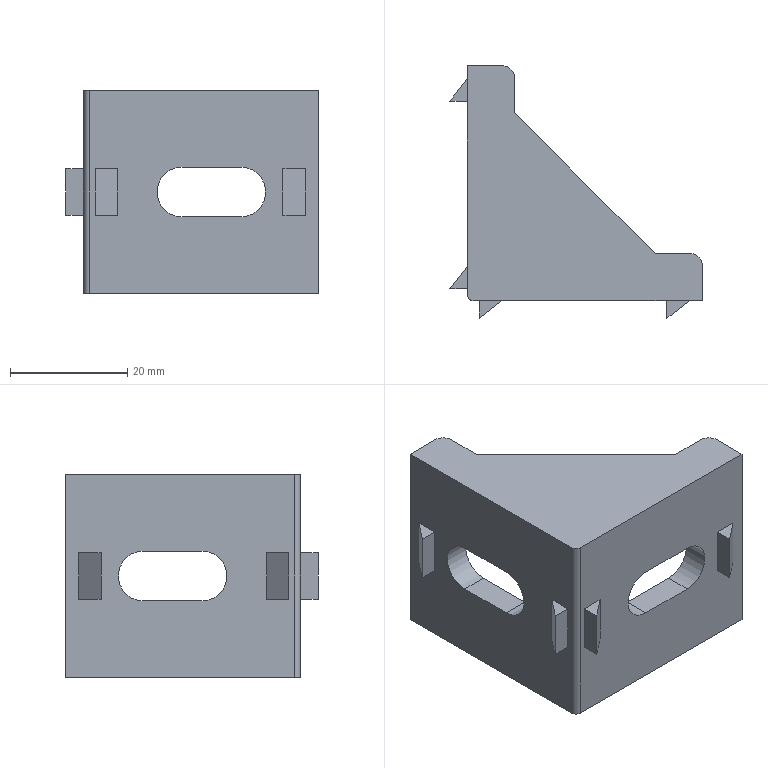Part | SolidWorks | features BaseBody 1 | 1 solid | 45 faces | box 43 x 43 x 34.5 mm | volume 13756 mm3 | plane 36 | cylinder 9 | commonest cylinder face diameters 4 x4 8.5 x4 2 x1
STEP:
#1=CARTESIAN_POINT('',(5.8,0.,-21.25));
#2=VERTEX_POINT('',#1);
#3=CARTESIAN_POINT('',(5.8,0.,-13.25));
#4=VERTEX_POINT('',#3);
#5=CARTESIAN_POINT('',(5.8,0.,-21.25));
#6=DIRECTION('',(0.,0.,1.));
#7=VECTOR('',#6,1000.);
#8=LINE('',#5,#7);
#9=EDGE_CURVE('',#2,#4,#8,.T.);
#10=ORIENTED_EDGE('',*,*,#9,.F.);
#11=CARTESIAN_POINT('',(2.,0.,-21.25));
#12=VERTEX_POINT('',#11);
#13=CARTESIAN_POINT('',(5.8,0.,-21.25));
#14=DIRECTION('',(1.,0.,0.));
#15=VECTOR('',#14,1000.);
#16=LINE('',#13,#15);
#17=EDGE_CURVE('',#12,#2,#16,.T.);
#18=ORIENTED_EDGE('',*,*,#17,.F.);
#19=CARTESIAN_POINT('',(2.,0.,-13.25));
#20=VERTEX_POINT('',#19);
#21=CARTESIAN_POINT('',(2.,0.,-21.25));
#22=DIRECTION('',(0.,0.,1.));
#23=VECTOR('',#22,1000.);
#24=LINE('',#21,#23);
#25=EDGE_CURVE('',#12,#20,#24,.T.);
#26=ORIENTED_EDGE('',*,*,#25,.T.);
#27=CARTESIAN_POINT('',(5.8,0.,-13.25));
#28=DIRECTION('',(1.,0.,0.));
#29=VECTOR('',#28,1000.);
#30=LINE('',#27,#29);
#31=EDGE_CURVE('',#20,#4,#30,.T.);
#32=ORIENTED_EDGE('',*,*,#31,.T.);
#33=EDGE_LOOP('',(#10,#18,#26,#32));
#34=FACE_BOUND('',#33,.T.);
#35=CARTESIAN_POINT('',(16.8,0.,-13.));
#36=VERTEX_POINT('',#35);
#37=CARTESIAN_POINT('',(16.8,0.,-21.5));
#38=VERTEX_POINT('',#37);
#39=CARTESIAN_POINT('',(16.8,0.,-17.25));
#40=DIRECTION('',(0.,-1.,0.));
#41=DIRECTION('',(0.,0.,-1.));
#42=AXIS2_PLACEMENT_3D('',#39,#40,#41);
#43=CIRCLE('',#42,4.25);
#44=EDGE_CURVE('',#36,#38,#43,.T.);
#45=ORIENTED_EDGE('',*,*,#44,.F.);
#46=CARTESIAN_POINT('',(26.8,0.,-13.));
#47=VERTEX_POINT('',#46);
#48=CARTESIAN_POINT('',(0.,0.,-13.));
#49=DIRECTION('',(-1.,0.,0.));
#50=VECTOR('',#49,1000.);
#51=LINE('',#48,#50);
#52=EDGE_CURVE('',#47,#36,#51,.T.);
#53=ORIENTED_EDGE('',*,*,#52,.F.);
#54=CARTESIAN_POINT('',(26.8,0.,-21.5));
#55=VERTEX_POINT('',#54);
#56=CARTESIAN_POINT('',(26.8,0.,-17.25));
#57=DIRECTION('',(0.,-1.,0.));
#58=DIRECTION('',(0.,0.,-1.));
#59=AXIS2_PLACEMENT_3D('',#56,#57,#58);
#60=CIRCLE('',#59,4.25);
#61=EDGE_CURVE('',#55,#47,#60,.T.);
#62=ORIENTED_EDGE('',*,*,#61,.F.);
#63=CARTESIAN_POINT('',(0.,0.,-21.5));
#64=DIRECTION('',(1.,0.,0.));
#65=VECTOR('',#64,1000.);
#66=LINE('',#63,#65);
#67=EDGE_CURVE('',#38,#55,#66,.T.);
#68=ORIENTED_EDGE('',*,*,#67,.F.);
#69=EDGE_LOOP('',(#45,#53,#62,#68));
#70=FACE_BOUND('',#69,.T.);
#71=CARTESIAN_POINT('',(1.,0.,0.));
#72=VERTEX_POINT('',#71);
#73=CARTESIAN_POINT('',(40.,0.,0.));
#74=VERTEX_POINT('',#73);
#75=CARTESIAN_POINT('',(0.,0.,0.));
#76=DIRECTION('',(1.,0.,0.));
#77=VECTOR('',#76,1000.);
#78=LINE('',#75,#77);
#79=EDGE_CURVE('',#72,#74,#78,.T.);
#80=ORIENTED_EDGE('',*,*,#79,.F.);
#81=CARTESIAN_POINT('',(1.,0.,-34.5));
#82=VERTEX_POINT('',#81);
#83=CARTESIAN_POINT('',(1.,0.,-34.5));
#84=DIRECTION('',(0.,0.,-1.));
#85=VECTOR('',#84,1000.);
#86=LINE('',#83,#85);
#87=EDGE_CURVE('',#72,#82,#86,.T.);
#88=ORIENTED_EDGE('',*,*,#87,.T.);
#89=CARTESIAN_POINT('',(40.,0.,-34.5));
#90=VERTEX_POINT('',#89);
#91=CARTESIAN_POINT('',(0.,0.,-34.5));
#92=DIRECTION('',(1.,0.,0.));
#93=VECTOR('',#92,1000.);
#94=LINE('',#91,#93);
#95=EDGE_CURVE('',#82,#90,#94,.T.);
#96=ORIENTED_EDGE('',*,*,#95,.T.);
#97=CARTESIAN_POINT('',(40.,0.,-34.5));
#98=DIRECTION('',(0.,0.,1.));
#99=VECTOR('',#98,1000.);
#100=LINE('',#97,#99);
#101=EDGE_CURVE('',#90,#74,#100,.T.);
#102=ORIENTED_EDGE('',*,*,#101,.T.);
#103=EDGE_LOOP('',(#80,#88,#96,#102));
#104=FACE_OUTER_BOUND('',#103,.T.);
#105=CARTESIAN_POINT('',(37.8,0.,-21.25));
#106=VERTEX_POINT('',#105);
#107=CARTESIAN_POINT('',(37.8,0.,-13.25));
#108=VERTEX_POINT('',#107);
#109=CARTESIAN_POINT('',(37.8,0.,-21.25));
#110=DIRECTION('',(0.,0.,1.));
#111=VECTOR('',#110,1000.);
#112=LINE('',#109,#111);
#113=EDGE_CURVE('',#106,#108,#112,.T.);
#114=ORIENTED_EDGE('',*,*,#113,.F.);
#115=CARTESIAN_POINT('',(34.,0.,-21.25));
#116=VERTEX_POINT('',#115);
#117=CARTESIAN_POINT('',(34.,0.,-21.25));
#118=DIRECTION('',(1.,0.,0.));
#119=VECTOR('',#118,1000.);
#120=LINE('',#117,#119);
#121=EDGE_CURVE('',#116,#106,#120,.T.);
#122=ORIENTED_EDGE('',*,*,#121,.F.);
#123=CARTESIAN_POINT('',(34.,0.,-13.25));
#124=VERTEX_POINT('',#123);
#125=CARTESIAN_POINT('',(34.,0.,-21.25));
#126=DIRECTION('',(0.,0.,1.));
#127=VECTOR('',#126,1000.);
#128=LINE('',#125,#127);
#129=EDGE_CURVE('',#116,#124,#128,.T.);
#130=ORIENTED_EDGE('',*,*,#129,.T.);
#131=CARTESIAN_POINT('',(34.,0.,-13.25));
#132=DIRECTION('',(1.,0.,0.));
#133=VECTOR('',#132,1000.);
#134=LINE('',#131,#133);
#135=EDGE_CURVE('',#124,#108,#134,.T.);
#136=ORIENTED_EDGE('',*,*,#135,.T.);
#137=EDGE_LOOP('',(#114,#122,#130,#136));
#138=FACE_BOUND('',#137,.T.);
#139=CARTESIAN_POINT('',(0.,0.,-34.5));
#140=DIRECTION('',(0.,-1.,0.));
#141=DIRECTION('',(0.,0.,-1.));
#142=AXIS2_PLACEMENT_3D('',#139,#140,#141);
#143=PLANE('',#142);
#144=ADVANCED_FACE('',(#34,#70,#104,#138),#143,.T.);
#145=CARTESIAN_POINT('',(4.5,26.8,-21.5));
#146=VERTEX_POINT('',#145);
#147=CARTESIAN_POINT('',(4.5,26.8,-13.));
#148=VERTEX_POINT('',#147);
#149=CARTESIAN_POINT('',(4.5,26.8,-17.25));
#150=DIRECTION('',(1.,0.,0.));
#151=DIRECTION('',(0.,0.,-1.));
#152=AXIS2_PLACEMENT_3D('',#149,#150,#151);
#153=CIRCLE('',#152,4.25);
#154=EDGE_CURVE('',#146,#148,#153,.T.);
#155=ORIENTED_EDGE('',*,*,#154,.F.);
#156=CARTESIAN_POINT('',(4.5,16.8,-21.5));
#157=VERTEX_POINT('',#156);
#158=CARTESIAN_POINT('',(4.5,26.8,-21.5));
#159=DIRECTION('',(0.,1.,0.));
#160=VECTOR('',#159,1000.);
#161=LINE('',#158,#160);
#162=EDGE_CURVE('',#157,#146,#161,.T.);
#163=ORIENTED_EDGE('',*,*,#162,.F.);
#164=CARTESIAN_POINT('',(4.5,16.8,-13.));
#165=VERTEX_POINT('',#164);
#166=CARTESIAN_POINT('',(4.5,16.8,-17.25));
#167=DIRECTION('',(1.,0.,0.));
#168=DIRECTION('',(0.,0.,-1.));
#169=AXIS2_PLACEMENT_3D('',#166,#167,#168);
#170=CIRCLE('',#169,4.25);
#171=EDGE_CURVE('',#165,#157,#170,.T.);
#172=ORIENTED_EDGE('',*,*,#171,.F.);
#173=CARTESIAN_POINT('',(4.5,26.8,-13.));
#174=DIRECTION('',(0.,-1.,0.));
#175=VECTOR('',#174,1000.);
#176=LINE('',#173,#175);
#177=EDGE_CURVE('',#148,#165,#176,.T.);
#178=ORIENTED_EDGE('',*,*,#177,.F.);
#179=EDGE_LOOP('',(#155,#163,#172,#178));
#180=FACE_BOUND('',#179,.T.);
#181=CARTESIAN_POINT('',(4.5,4.5,-31.5));
#182=VERTEX_POINT('',#181);
#183=CARTESIAN_POINT('',(4.5,4.5,-3.));
#184=VERTEX_POINT('',#183);
#185=CARTESIAN_POINT('',(4.5,4.5,-34.5));
#186=DIRECTION('',(0.,0.,1.));
#187=VECTOR('',#186,1000.);
#188=LINE('',#185,#187);
#189=EDGE_CURVE('',#182,#184,#188,.T.);
#190=ORIENTED_EDGE('',*,*,#189,.F.);
#191=CARTESIAN_POINT('',(4.5,40.,-31.5));
#192=VERTEX_POINT('',#191);
#193=CARTESIAN_POINT('',(4.5,40.,-31.5));
#194=DIRECTION('',(0.,-1.,0.));
#195=VECTOR('',#194,1000.);
#196=LINE('',#193,#195);
#197=EDGE_CURVE('',#192,#182,#196,.T.);
#198=ORIENTED_EDGE('',*,*,#197,.F.);
#199=CARTESIAN_POINT('',(4.5,40.,-3.));
#200=VERTEX_POINT('',#199);
#201=CARTESIAN_POINT('',(4.5,40.,-34.5));
#202=DIRECTION('',(0.,0.,1.));
#203=VECTOR('',#202,1000.);
#204=LINE('',#201,#203);
#205=EDGE_CURVE('',#192,#200,#204,.T.);
#206=ORIENTED_EDGE('',*,*,#205,.T.);
#207=CARTESIAN_POINT('',(4.5,40.,-3.));
#208=DIRECTION('',(0.,-1.,0.));
#209=VECTOR('',#208,1000.);
#210=LINE('',#207,#209);
#211=EDGE_CURVE('',#200,#184,#210,.T.);
#212=ORIENTED_EDGE('',*,*,#211,.T.);
#213=EDGE_LOOP('',(#190,#198,#206,#212));
#214=FACE_OUTER_BOUND('',#213,.T.);
#215=CARTESIAN_POINT('',(4.5,4.5,-34.5));
#216=DIRECTION('',(1.,0.,0.));
#217=DIRECTION('',(0.,0.,-1.));
#218=AXIS2_PLACEMENT_3D('',#215,#216,#217);
#219=PLANE('',#218);
#220=ADVANCED_FACE('',(#180,#214),#219,.T.);
#221=CARTESIAN_POINT('',(16.8,4.5,-21.5));
#222=VERTEX_POINT('',#221);
#223=CARTESIAN_POINT('',(16.8,4.5,-13.));
#224=VERTEX_POINT('',#223);
#225=CARTESIAN_POINT('',(16.8,4.5,-17.25));
#226=DIRECTION('',(0.,1.,0.));
#227=DIRECTION('',(0.,0.,1.));
#228=AXIS2_PLACEMENT_3D('',#225,#226,#227);
#229=CIRCLE('',#228,4.25);
#230=EDGE_CURVE('',#222,#224,#229,.T.);
#231=ORIENTED_EDGE('',*,*,#230,.F.);
#232=CARTESIAN_POINT('',(26.8,4.5,-21.5));
#233=VERTEX_POINT('',#232);
#234=CARTESIAN_POINT('',(16.8,4.5,-21.5));
#235=DIRECTION('',(-1.,0.,0.));
#236=VECTOR('',#235,1000.);
#237=LINE('',#234,#236);
#238=EDGE_CURVE('',#233,#222,#237,.T.);
#239=ORIENTED_EDGE('',*,*,#238,.F.);
#240=CARTESIAN_POINT('',(26.8,4.5,-13.));
#241=VERTEX_POINT('',#240);
#242=CARTESIAN_POINT('',(26.8,4.5,-17.25));
#243=DIRECTION('',(0.,1.,0.));
#244=DIRECTION('',(0.,0.,1.));
#245=AXIS2_PLACEMENT_3D('',#242,#243,#244);
#246=CIRCLE('',#245,4.25);
#247=EDGE_CURVE('',#241,#233,#246,.T.);
#248=ORIENTED_EDGE('',*,*,#247,.F.);
#249=CARTESIAN_POINT('',(16.8,4.5,-13.));
#250=DIRECTION('',(1.,0.,0.));
#251=VECTOR('',#250,1000.);
#252=LINE('',#249,#251);
#253=EDGE_CURVE('',#224,#241,#252,.T.);
#254=ORIENTED_EDGE('',*,*,#253,.F.);
#255=EDGE_LOOP('',(#231,#239,#248,#254));
#256=FACE_BOUND('',#255,.T.);
#257=CARTESIAN_POINT('',(40.,4.5,-31.5));
#258=VERTEX_POINT('',#257);
#259=CARTESIAN_POINT('',(40.,4.5,-3.));
#260=VERTEX_POINT('',#259);
#261=CARTESIAN_POINT('',(40.,4.5,-34.5));
#262=DIRECTION('',(0.,0.,1.));
#263=VECTOR('',#262,1000.);
#264=LINE('',#261,#263);
#265=EDGE_CURVE('',#258,#260,#264,.T.);
#266=ORIENTED_EDGE('',*,*,#265,.F.);
#267=CARTESIAN_POINT('',(4.5,4.5,-31.5));
#268=DIRECTION('',(1.,0.,0.));
#269=VECTOR('',#268,1000.);
#270=LINE('',#267,#269);
#271=EDGE_CURVE('',#182,#258,#270,.T.);
#272=ORIENTED_EDGE('',*,*,#271,.F.);
#273=ORIENTED_EDGE('',*,*,#189,.T.);
#274=CARTESIAN_POINT('',(4.5,4.5,-3.));
#275=DIRECTION('',(1.,0.,0.));
#276=VECTOR('',#275,1000.);
#277=LINE('',#274,#276);
#278=EDGE_CURVE('',#184,#260,#277,.T.);
#279=ORIENTED_EDGE('',*,*,#278,.T.);
#280=EDGE_LOOP('',(#266,#272,#273,#279));
#281=FACE_OUTER_BOUND('',#280,.T.);
#282=CARTESIAN_POINT('',(4.5,4.5,-34.5));
#283=DIRECTION('',(0.,1.,0.));
#284=DIRECTION('',(0.,0.,1.));
#285=AXIS2_PLACEMENT_3D('',#282,#283,#284);
#286=PLANE('',#285);
#287=ADVANCED_FACE('',(#256,#281),#286,.T.);
#288=CARTESIAN_POINT('',(0.,5.8,-21.25));
#289=VERTEX_POINT('',#288);
#290=CARTESIAN_POINT('',(0.,2.,-21.25));
#291=VERTEX_POINT('',#290);
#292=CARTESIAN_POINT('',(0.,5.8,-21.25));
#293=DIRECTION('',(0.,-1.,0.));
#294=VECTOR('',#293,1000.);
#295=LINE('',#292,#294);
#296=EDGE_CURVE('',#289,#291,#295,.T.);
#297=ORIENTED_EDGE('',*,*,#296,.F.);
#298=CARTESIAN_POINT('',(0.,5.8,-13.25));
#299=VERTEX_POINT('',#298);
#300=CARTESIAN_POINT('',(0.,5.8,-21.25));
#301=DIRECTION('',(0.,0.,1.));
#302=VECTOR('',#301,1000.);
#303=LINE('',#300,#302);
#304=EDGE_CURVE('',#289,#299,#303,.T.);
#305=ORIENTED_EDGE('',*,*,#304,.T.);
#306=CARTESIAN_POINT('',(0.,2.,-13.25));
#307=VERTEX_POINT('',#306);
#308=CARTESIAN_POINT('',(0.,5.8,-13.25));
#309=DIRECTION('',(0.,-1.,0.));
#310=VECTOR('',#309,1000.);
#311=LINE('',#308,#310);
#312=EDGE_CURVE('',#299,#307,#311,.T.);
#313=ORIENTED_EDGE('',*,*,#312,.T.);
#314=CARTESIAN_POINT('',(0.,2.,-21.25));
#315=DIRECTION('',(0.,0.,1.));
#316=VECTOR('',#315,1000.);
#317=LINE('',#314,#316);
#318=EDGE_CURVE('',#291,#307,#317,.T.);
#319=ORIENTED_EDGE('',*,*,#318,.F.);
#320=EDGE_LOOP('',(#297,#305,#313,#319));
#321=FACE_BOUND('',#320,.T.);
#322=CARTESIAN_POINT('',(0.,37.8,-21.25));
#323=VERTEX_POINT('',#322);
#324=CARTESIAN_POINT('',(0.,34.,-21.25));
#325=VERTEX_POINT('',#324);
#326=CARTESIAN_POINT('',(0.,37.8,-21.25));
#327=DIRECTION('',(0.,-1.,0.));
#328=VECTOR('',#327,1000.);
#329=LINE('',#326,#328);
#330=EDGE_CURVE('',#323,#325,#329,.T.);
#331=ORIENTED_EDGE('',*,*,#330,.F.);
#332=CARTESIAN_POINT('',(0.,37.8,-13.25));
#333=VERTEX_POINT('',#332);
#334=CARTESIAN_POINT('',(0.,37.8,-21.25));
#335=DIRECTION('',(0.,0.,1.));
#336=VECTOR('',#335,1000.);
#337=LINE('',#334,#336);
#338=EDGE_CURVE('',#323,#333,#337,.T.);
#339=ORIENTED_EDGE('',*,*,#338,.T.);
#340=CARTESIAN_POINT('',(0.,34.,-13.25));
#341=VERTEX_POINT('',#340);
#342=CARTESIAN_POINT('',(0.,37.8,-13.25));
#343=DIRECTION('',(0.,-1.,0.));
#344=VECTOR('',#343,1000.);
#345=LINE('',#342,#344);
#346=EDGE_CURVE('',#333,#341,#345,.T.);
#347=ORIENTED_EDGE('',*,*,#346,.T.);
#348=CARTESIAN_POINT('',(0.,34.,-21.25));
#349=DIRECTION('',(0.,0.,1.));
#350=VECTOR('',#349,1000.);
#351=LINE('',#348,#350);
#352=EDGE_CURVE('',#325,#341,#351,.T.);
#353=ORIENTED_EDGE('',*,*,#352,.F.);
#354=EDGE_LOOP('',(#331,#339,#347,#353));
#355=FACE_BOUND('',#354,.T.);
#356=CARTESIAN_POINT('',(0.,26.8,-13.));
#357=VERTEX_POINT('',#356);
#358=CARTESIAN_POINT('',(0.,26.8,-21.5));
#359=VERTEX_POINT('',#358);
#360=CARTESIAN_POINT('',(0.,26.8,-17.25));
#361=DIRECTION('',(-1.,0.,0.));
#362=DIRECTION('',(0.,0.,1.));
#363=AXIS2_PLACEMENT_3D('',#360,#361,#362);
#364=CIRCLE('',#363,4.25);
#365=EDGE_CURVE('',#357,#359,#364,.T.);
#366=ORIENTED_EDGE('',*,*,#365,.F.);
#367=CARTESIAN_POINT('',(0.,16.8,-13.));
#368=VERTEX_POINT('',#367);
#369=CARTESIAN_POINT('',(0.,0.,-13.));
#370=DIRECTION('',(0.,1.,0.));
#371=VECTOR('',#370,1000.);
#372=LINE('',#369,#371);
#373=EDGE_CURVE('',#368,#357,#372,.T.);
#374=ORIENTED_EDGE('',*,*,#373,.F.);
#375=CARTESIAN_POINT('',(0.,16.8,-21.5));
#376=VERTEX_POINT('',#375);
#377=CARTESIAN_POINT('',(0.,16.8,-17.25));
#378=DIRECTION('',(-1.,0.,0.));
#379=DIRECTION('',(0.,0.,1.));
#380=AXIS2_PLACEMENT_3D('',#377,#378,#379);
#381=CIRCLE('',#380,4.25);
#382=EDGE_CURVE('',#376,#368,#381,.T.);
#383=ORIENTED_EDGE('',*,*,#382,.F.);
#384=CARTESIAN_POINT('',(0.,0.,-21.5));
#385=DIRECTION('',(0.,-1.,0.));
#386=VECTOR('',#385,1000.);
#387=LINE('',#384,#386);
#388=EDGE_CURVE('',#359,#376,#387,.T.);
#389=ORIENTED_EDGE('',*,*,#388,.F.);
#390=EDGE_LOOP('',(#366,#374,#383,#389));
#391=FACE_BOUND('',#390,.T.);
#392=CARTESIAN_POINT('',(0.,40.,-34.5));
#393=VERTEX_POINT('',#392);
#394=CARTESIAN_POINT('',(0.,1.,-34.5));
#395=VERTEX_POINT('',#394);
#396=CARTESIAN_POINT('',(0.,0.,-34.5));
#397=DIRECTION('',(0.,-1.,0.));
#398=VECTOR('',#397,1000.);
#399=LINE('',#396,#398);
#400=EDGE_CURVE('',#393,#395,#399,.T.);
#401=ORIENTED_EDGE('',*,*,#400,.T.);
#402=CARTESIAN_POINT('',(0.,1.,0.));
#403=VERTEX_POINT('',#402);
#404=CARTESIAN_POINT('',(0.,1.,-34.5));
#405=DIRECTION('',(0.,0.,1.));
#406=VECTOR('',#405,1000.);
#407=LINE('',#404,#406);
#408=EDGE_CURVE('',#395,#403,#407,.T.);
#409=ORIENTED_EDGE('',*,*,#408,.T.);
#410=CARTESIAN_POINT('',(0.,40.,0.));
#411=VERTEX_POINT('',#410);
#412=CARTESIAN_POINT('',(0.,0.,0.));
#413=DIRECTION('',(0.,-1.,0.));
#414=VECTOR('',#413,1000.);
#415=LINE('',#412,#414);
#416=EDGE_CURVE('',#411,#403,#415,.T.);
#417=ORIENTED_EDGE('',*,*,#416,.F.);
#418=CARTESIAN_POINT('',(0.,40.,-34.5));
#419=DIRECTION('',(0.,0.,1.));
#420=VECTOR('',#419,1000.);
#421=LINE('',#418,#420);
#422=EDGE_CURVE('',#393,#411,#421,.T.);
#423=ORIENTED_EDGE('',*,*,#422,.F.);
#424=EDGE_LOOP('',(#401,#409,#417,#423));
#425=FACE_OUTER_BOUND('',#424,.T.);
#426=CARTESIAN_POINT('',(0.,0.,-34.5));
#427=DIRECTION('',(-1.,0.,0.));
#428=DIRECTION('',(0.,0.,1.));
#429=AXIS2_PLACEMENT_3D('',#426,#427,#428);
#430=PLANE('',#429);
#431=ADVANCED_FACE('',(#321,#355,#391,#425),#430,.T.);
#432=CARTESIAN_POINT('',(6.,40.,0.));
#433=VERTEX_POINT('',#432);
#434=CARTESIAN_POINT('',(0.,40.,0.));
#435=DIRECTION('',(-1.,0.,0.));
#436=VECTOR('',#435,1000.);
#437=LINE('',#434,#436);
#438=EDGE_CURVE('',#433,#411,#437,.T.);
#439=ORIENTED_EDGE('',*,*,#438,.F.);
#440=CARTESIAN_POINT('',(6.,40.,-3.));
#441=VERTEX_POINT('',#440);
#442=CARTESIAN_POINT('',(6.,40.,-34.5));
#443=DIRECTION('',(0.,0.,-1.));
#444=VECTOR('',#443,1000.);
#445=LINE('',#442,#444);
#446=EDGE_CURVE('',#433,#441,#445,.T.);
#447=ORIENTED_EDGE('',*,*,#446,.T.);
#448=CARTESIAN_POINT('',(4.5,40.,-3.));
#449=DIRECTION('',(-1.,0.,0.));
#450=VECTOR('',#449,1000.);
#451=LINE('',#448,#450);
#452=EDGE_CURVE('',#441,#200,#451,.T.);
#453=ORIENTED_EDGE('',*,*,#452,.T.);
#454=ORIENTED_EDGE('',*,*,#205,.F.);
#455=CARTESIAN_POINT('',(6.,40.,-31.5));
#456=VERTEX_POINT('',#455);
#457=CARTESIAN_POINT('',(4.5,40.,-31.5));
#458=DIRECTION('',(-1.,0.,0.));
#459=VECTOR('',#458,1000.);
#460=LINE('',#457,#459);
#461=EDGE_CURVE('',#456,#192,#460,.T.);
#462=ORIENTED_EDGE('',*,*,#461,.F.);
#463=CARTESIAN_POINT('',(6.,40.,-34.5));
#464=VERTEX_POINT('',#463);
#465=CARTESIAN_POINT('',(6.,40.,-34.5));
#466=DIRECTION('',(0.,0.,-1.));
#467=VECTOR('',#466,1000.);
#468=LINE('',#465,#467);
#469=EDGE_CURVE('',#456,#464,#468,.T.);
#470=ORIENTED_EDGE('',*,*,#469,.T.);
#471=CARTESIAN_POINT('',(0.,40.,-34.5));
#472=DIRECTION('',(-1.,0.,0.));
#473=VECTOR('',#472,1000.);
#474=LINE('',#471,#473);
#475=EDGE_CURVE('',#464,#393,#474,.T.);
#476=ORIENTED_EDGE('',*,*,#475,.T.);
#477=ORIENTED_EDGE('',*,*,#422,.T.);
#478=EDGE_LOOP('',(#439,#447,#453,#454,#462,#470,#476,#477));
#479=FACE_OUTER_BOUND('',#478,.T.);
#480=CARTESIAN_POINT('',(0.,40.,-34.5));
#481=DIRECTION('',(0.,1.,0.));
#482=DIRECTION('',(0.,0.,1.));
#483=AXIS2_PLACEMENT_3D('',#480,#481,#482);
#484=PLANE('',#483);
#485=ADVANCED_FACE('',(#479),#484,.T.);
#486=CARTESIAN_POINT('',(40.,6.,-3.));
#487=VERTEX_POINT('',#486);
#488=CARTESIAN_POINT('',(40.,8.,-3.));
#489=DIRECTION('',(0.,1.,0.));
#490=VECTOR('',#489,1000.);
#491=LINE('',#488,#490);
#492=EDGE_CURVE('',#260,#487,#491,.T.);
#493=ORIENTED_EDGE('',*,*,#492,.T.);
#494=CARTESIAN_POINT('',(40.,6.,0.));
#495=VERTEX_POINT('',#494);
#496=CARTESIAN_POINT('',(40.,6.,-34.5));
#497=DIRECTION('',(0.,0.,1.));
#498=VECTOR('',#497,1000.);
#499=LINE('',#496,#498);
#500=EDGE_CURVE('',#487,#495,#499,.T.);
#501=ORIENTED_EDGE('',*,*,#500,.T.);
#502=CARTESIAN_POINT('',(40.,4.5,0.));
#503=DIRECTION('',(0.,1.,0.));
#504=VECTOR('',#503,1000.);
#505=LINE('',#502,#504);
#506=EDGE_CURVE('',#74,#495,#505,.T.);
#507=ORIENTED_EDGE('',*,*,#506,.F.);
#508=ORIENTED_EDGE('',*,*,#101,.F.);
#509=CARTESIAN_POINT('',(40.,6.,-34.5));
#510=VERTEX_POINT('',#509);
#511=CARTESIAN_POINT('',(40.,4.5,-34.5));
#512=DIRECTION('',(0.,1.,0.));
#513=VECTOR('',#512,1000.);
#514=LINE('',#511,#513);
#515=EDGE_CURVE('',#90,#510,#514,.T.);
#516=ORIENTED_EDGE('',*,*,#515,.T.);
#517=CARTESIAN_POINT('',(40.,6.,-31.5));
#518=VERTEX_POINT('',#517);
#519=CARTESIAN_POINT('',(40.,6.,-31.5));
#520=DIRECTION('',(0.,0.,1.));
#521=VECTOR('',#520,1000.);
#522=LINE('',#519,#521);
#523=EDGE_CURVE('',#510,#518,#522,.T.);
#524=ORIENTED_EDGE('',*,*,#523,.T.);
#525=CARTESIAN_POINT('',(40.,8.,-31.5));
#526=DIRECTION('',(0.,1.,0.));
#527=VECTOR('',#526,1000.);
#528=LINE('',#525,#527);
#529=EDGE_CURVE('',#258,#518,#528,.T.);
#530=ORIENTED_EDGE('',*,*,#529,.F.);
#531=ORIENTED_EDGE('',*,*,#265,.T.);
#532=EDGE_LOOP('',(#493,#501,#507,#508,#516,#524,#530,#531));
#533=FACE_OUTER_BOUND('',#532,.T.);
#534=CARTESIAN_POINT('',(40.,4.5,-34.5));
#535=DIRECTION('',(1.,0.,0.));
#536=DIRECTION('',(0.,0.,-1.));
#537=AXIS2_PLACEMENT_3D('',#534,#535,#536);
#538=PLANE('',#537);
#539=ADVANCED_FACE('',(#533),#538,.T.);
#540=CARTESIAN_POINT('',(38.,8.,-34.5));
#541=VERTEX_POINT('',#540);
#542=CARTESIAN_POINT('',(32.,8.,-34.5));
#543=VERTEX_POINT('',#542);
#544=CARTESIAN_POINT('',(32.,8.,-34.5));
#545=DIRECTION('',(-1.,0.,0.));
#546=VECTOR('',#545,1000.);
#547=LINE('',#544,#546);
#548=EDGE_CURVE('',#541,#543,#547,.T.);
#549=ORIENTED_EDGE('',*,*,#548,.F.);
#550=CARTESIAN_POINT('',(38.,6.,-34.5));
#551=DIRECTION('',(0.,0.,-1.));
#552=DIRECTION('',(-1.,0.,0.));
#553=AXIS2_PLACEMENT_3D('',#550,#551,#552);
#554=CIRCLE('',#553,2.);
#555=EDGE_CURVE('',#541,#510,#554,.T.);
#556=ORIENTED_EDGE('',*,*,#555,.T.);
#557=ORIENTED_EDGE('',*,*,#515,.F.);
#558=ORIENTED_EDGE('',*,*,#95,.F.);
#559=CARTESIAN_POINT('',(1.,1.,-34.5));
#560=DIRECTION('',(0.,0.,-1.));
#561=DIRECTION('',(-1.,0.,0.));
#562=AXIS2_PLACEMENT_3D('',#559,#560,#561);
#563=CIRCLE('',#562,1.);
#564=EDGE_CURVE('',#82,#395,#563,.T.);
#565=ORIENTED_EDGE('',*,*,#564,.T.);
#566=ORIENTED_EDGE('',*,*,#400,.F.);
#567=ORIENTED_EDGE('',*,*,#475,.F.);
#568=CARTESIAN_POINT('',(8.,38.,-34.5));
#569=VERTEX_POINT('',#568);
#570=CARTESIAN_POINT('',(6.,38.,-34.5));
#571=DIRECTION('',(0.,0.,-1.));
#572=DIRECTION('',(-1.,0.,0.));
#573=AXIS2_PLACEMENT_3D('',#570,#571,#572);
#574=CIRCLE('',#573,2.);
#575=EDGE_CURVE('',#464,#569,#574,.T.);
#576=ORIENTED_EDGE('',*,*,#575,.T.);
#577=CARTESIAN_POINT('',(8.,32.,-34.5));
#578=VERTEX_POINT('',#577);
#579=CARTESIAN_POINT('',(8.,40.,-34.5));
#580=DIRECTION('',(0.,1.,0.));
#581=VECTOR('',#580,1000.);
#582=LINE('',#579,#581);
#583=EDGE_CURVE('',#578,#569,#582,.T.);
#584=ORIENTED_EDGE('',*,*,#583,.F.);
#585=CARTESIAN_POINT('',(8.,32.,-34.5));
#586=DIRECTION('',(-0.7071,0.7071,0.));
#587=VECTOR('',#586,1000.);
#588=LINE('',#585,#587);
#589=EDGE_CURVE('',#543,#578,#588,.T.);
#590=ORIENTED_EDGE('',*,*,#589,.F.);
#591=EDGE_LOOP('',(#549,#556,#557,#558,#565,#566,#567,#576,#584,#590));
#592=FACE_OUTER_BOUND('',#591,.T.);
#593=CARTESIAN_POINT('',(40.,0.,-34.5));
#594=DIRECTION('',(0.,0.,-1.));
#595=DIRECTION('',(-1.,0.,0.));
#596=AXIS2_PLACEMENT_3D('',#593,#594,#595);
#597=PLANE('',#596);
#598=ADVANCED_FACE('',(#592),#597,.T.);
#599=ORIENTED_EDGE('',*,*,#506,.T.);
#600=CARTESIAN_POINT('',(38.,8.,0.));
#601=VERTEX_POINT('',#600);
#602=CARTESIAN_POINT('',(38.,6.,0.));
#603=DIRECTION('',(0.,0.,1.));
#604=DIRECTION('',(-1.,0.,0.));
#605=AXIS2_PLACEMENT_3D('',#602,#603,#604);
#606=CIRCLE('',#605,2.);
#607=EDGE_CURVE('',#495,#601,#606,.T.);
#608=ORIENTED_EDGE('',*,*,#607,.T.);
#609=CARTESIAN_POINT('',(32.,8.,0.));
#610=VERTEX_POINT('',#609);
#611=CARTESIAN_POINT('',(32.,8.,0.));
#612=DIRECTION('',(-1.,0.,0.));
#613=VECTOR('',#612,1000.);
#614=LINE('',#611,#613);
#615=EDGE_CURVE('',#601,#610,#614,.T.);
#616=ORIENTED_EDGE('',*,*,#615,.T.);
#617=CARTESIAN_POINT('',(8.,32.,0.));
#618=VERTEX_POINT('',#617);
#619=CARTESIAN_POINT('',(8.,32.,0.));
#620=DIRECTION('',(-0.7071,0.7071,0.));
#621=VECTOR('',#620,1000.);
#622=LINE('',#619,#621);
#623=EDGE_CURVE('',#610,#618,#622,.T.);
#624=ORIENTED_EDGE('',*,*,#623,.T.);
#625=CARTESIAN_POINT('',(8.,38.,0.));
#626=VERTEX_POINT('',#625);
#627=CARTESIAN_POINT('',(8.,40.,0.));
#628=DIRECTION('',(0.,1.,0.));
#629=VECTOR('',#628,1000.);
#630=LINE('',#627,#629);
#631=EDGE_CURVE('',#618,#626,#630,.T.);
#632=ORIENTED_EDGE('',*,*,#631,.T.);
#633=CARTESIAN_POINT('',(6.,38.,0.));
#634=DIRECTION('',(0.,0.,1.));
#635=DIRECTION('',(-1.,0.,0.));
#636=AXIS2_PLACEMENT_3D('',#633,#634,#635);
#637=CIRCLE('',#636,2.);
#638=EDGE_CURVE('',#626,#433,#637,.T.);
#639=ORIENTED_EDGE('',*,*,#638,.T.);
#640=ORIENTED_EDGE('',*,*,#438,.T.);
#641=ORIENTED_EDGE('',*,*,#416,.T.);
#642=CARTESIAN_POINT('',(1.,1.,0.));
#643=DIRECTION('',(0.,0.,1.));
#644=DIRECTION('',(-1.,0.,0.));
#645=AXIS2_PLACEMENT_3D('',#642,#643,#644);
#646=CIRCLE('',#645,1.);
#647=EDGE_CURVE('',#403,#72,#646,.T.);
#648=ORIENTED_EDGE('',*,*,#647,.T.);
#649=ORIENTED_EDGE('',*,*,#79,.T.);
#650=EDGE_LOOP('',(#599,#608,#616,#624,#632,#639,#640,#641,#648,#649));
#651=FACE_OUTER_BOUND('',#650,.T.);
#652=CARTESIAN_POINT('',(40.,0.,0.));
#653=DIRECTION('',(0.,0.,-1.));
#654=DIRECTION('',(-1.,0.,0.));
#655=AXIS2_PLACEMENT_3D('',#652,#653,#654);
#656=PLANE('',#655);
#657=ADVANCED_FACE('',(#651),#656,.F.);
#658=ORIENTED_EDGE('',*,*,#44,.T.);
#659=CARTESIAN_POINT('',(16.8,-23.5,-21.5));
#660=DIRECTION('',(0.,1.,0.));
#661=VECTOR('',#660,1000.);
#662=LINE('',#659,#661);
#663=EDGE_CURVE('',#38,#222,#662,.T.);
#664=ORIENTED_EDGE('',*,*,#663,.T.);
#665=ORIENTED_EDGE('',*,*,#230,.T.);
#666=CARTESIAN_POINT('',(16.8,-23.5,-13.));
#667=DIRECTION('',(0.,1.,0.));
#668=VECTOR('',#667,1000.);
#669=LINE('',#666,#668);
#670=EDGE_CURVE('',#36,#224,#669,.T.);
#671=ORIENTED_EDGE('',*,*,#670,.F.);
#672=EDGE_LOOP('',(#658,#664,#665,#671));
#673=FACE_OUTER_BOUND('',#672,.T.);
#674=CARTESIAN_POINT('',(16.8,-23.5,-17.25));
#675=DIRECTION('',(0.,1.,0.));
#676=DIRECTION('',(0.,0.,1.));
#677=AXIS2_PLACEMENT_3D('',#674,#675,#676);
#678=CYLINDRICAL_SURFACE('',#677,4.25);
#679=ADVANCED_FACE('',(#673),#678,.F.);
#680=ORIENTED_EDGE('',*,*,#67,.T.);
#681=CARTESIAN_POINT('',(26.8,-23.5,-21.5));
#682=DIRECTION('',(0.,1.,0.));
#683=VECTOR('',#682,1000.);
#684=LINE('',#681,#683);
#685=EDGE_CURVE('',#55,#233,#684,.T.);
#686=ORIENTED_EDGE('',*,*,#685,.T.);
#687=ORIENTED_EDGE('',*,*,#238,.T.);
#688=ORIENTED_EDGE('',*,*,#663,.F.);
#689=EDGE_LOOP('',(#680,#686,#687,#688));
#690=FACE_OUTER_BOUND('',#689,.T.);
#691=CARTESIAN_POINT('',(16.8,-23.5,-21.5));
#692=DIRECTION('',(0.,0.,-1.));
#693=DIRECTION('',(-1.,0.,0.));
#694=AXIS2_PLACEMENT_3D('',#691,#692,#693);
#695=PLANE('',#694);
#696=ADVANCED_FACE('',(#690),#695,.F.);
#697=ORIENTED_EDGE('',*,*,#61,.T.);
#698=CARTESIAN_POINT('',(26.8,-23.5,-13.));
#699=DIRECTION('',(0.,1.,0.));
#700=VECTOR('',#699,1000.);
#701=LINE('',#698,#700);
#702=EDGE_CURVE('',#47,#241,#701,.T.);
#703=ORIENTED_EDGE('',*,*,#702,.T.);
#704=ORIENTED_EDGE('',*,*,#247,.T.);
#705=ORIENTED_EDGE('',*,*,#685,.F.);
#706=EDGE_LOOP('',(#697,#703,#704,#705));
#707=FACE_OUTER_BOUND('',#706,.T.);
#708=CARTESIAN_POINT('',(26.8,-23.5,-17.25));
#709=DIRECTION('',(0.,1.,0.));
#710=DIRECTION('',(0.,0.,1.));
#711=AXIS2_PLACEMENT_3D('',#708,#709,#710);
#712=CYLINDRICAL_SURFACE('',#711,4.25);
#713=ADVANCED_FACE('',(#707),#712,.F.);
#714=ORIENTED_EDGE('',*,*,#52,.T.);
#715=ORIENTED_EDGE('',*,*,#670,.T.);
#716=ORIENTED_EDGE('',*,*,#253,.T.);
#717=ORIENTED_EDGE('',*,*,#702,.F.);
#718=EDGE_LOOP('',(#714,#715,#716,#717));
#719=FACE_OUTER_BOUND('',#718,.T.);
#720=CARTESIAN_POINT('',(16.8,-23.5,-13.));
#721=DIRECTION('',(0.,0.,1.));
#722=DIRECTION('',(1.,0.,0.));
#723=AXIS2_PLACEMENT_3D('',#720,#721,#722);
#724=PLANE('',#723);
#725=ADVANCED_FACE('',(#719),#724,.F.);
#726=ORIENTED_EDGE('',*,*,#365,.T.);
#727=CARTESIAN_POINT('',(-23.5,26.8,-21.5));
#728=DIRECTION('',(1.,0.,0.));
#729=VECTOR('',#728,1000.);
#730=LINE('',#727,#729);
#731=EDGE_CURVE('',#359,#146,#730,.T.);
#732=ORIENTED_EDGE('',*,*,#731,.T.);
#733=ORIENTED_EDGE('',*,*,#154,.T.);
#734=CARTESIAN_POINT('',(-23.5,26.8,-13.));
#735=DIRECTION('',(1.,0.,0.));
#736=VECTOR('',#735,1000.);
#737=LINE('',#734,#736);
#738=EDGE_CURVE('',#357,#148,#737,.T.);
#739=ORIENTED_EDGE('',*,*,#738,.F.);
#740=EDGE_LOOP('',(#726,#732,#733,#739));
#741=FACE_OUTER_BOUND('',#740,.T.);
#742=CARTESIAN_POINT('',(-23.5,26.8,-17.25));
#743=DIRECTION('',(1.,0.,0.));
#744=DIRECTION('',(0.,0.,-1.));
#745=AXIS2_PLACEMENT_3D('',#742,#743,#744);
#746=CYLINDRICAL_SURFACE('',#745,4.25);
#747=ADVANCED_FACE('',(#741),#746,.F.);
#748=ORIENTED_EDGE('',*,*,#388,.T.);
#749=CARTESIAN_POINT('',(-23.5,16.8,-21.5));
#750=DIRECTION('',(1.,0.,0.));
#751=VECTOR('',#750,1000.);
#752=LINE('',#749,#751);
#753=EDGE_CURVE('',#376,#157,#752,.T.);
#754=ORIENTED_EDGE('',*,*,#753,.T.);
#755=ORIENTED_EDGE('',*,*,#162,.T.);
#756=ORIENTED_EDGE('',*,*,#731,.F.);
#757=EDGE_LOOP('',(#748,#754,#755,#756));
#758=FACE_OUTER_BOUND('',#757,.T.);
#759=CARTESIAN_POINT('',(-23.5,26.8,-21.5));
#760=DIRECTION('',(0.,0.,-1.));
#761=DIRECTION('',(-1.,0.,0.));
#762=AXIS2_PLACEMENT_3D('',#759,#760,#761);
#763=PLANE('',#762);
#764=ADVANCED_FACE('',(#758),#763,.F.);
#765=ORIENTED_EDGE('',*,*,#382,.T.);
#766=CARTESIAN_POINT('',(-23.5,16.8,-13.));
#767=DIRECTION('',(1.,0.,0.));
#768=VECTOR('',#767,1000.);
#769=LINE('',#766,#768);
#770=EDGE_CURVE('',#368,#165,#769,.T.);
#771=ORIENTED_EDGE('',*,*,#770,.T.);
#772=ORIENTED_EDGE('',*,*,#171,.T.);
#773=ORIENTED_EDGE('',*,*,#753,.F.);
#774=EDGE_LOOP('',(#765,#771,#772,#773));
#775=FACE_OUTER_BOUND('',#774,.T.);
#776=CARTESIAN_POINT('',(-23.5,16.8,-17.25));
#777=DIRECTION('',(1.,0.,0.));
#778=DIRECTION('',(0.,0.,-1.));
#779=AXIS2_PLACEMENT_3D('',#776,#777,#778);
#780=CYLINDRICAL_SURFACE('',#779,4.25);
#781=ADVANCED_FACE('',(#775),#780,.F.);
#782=ORIENTED_EDGE('',*,*,#373,.T.);
#783=ORIENTED_EDGE('',*,*,#738,.T.);
#784=ORIENTED_EDGE('',*,*,#177,.T.);
#785=ORIENTED_EDGE('',*,*,#770,.F.);
#786=EDGE_LOOP('',(#782,#783,#784,#785));
#787=FACE_OUTER_BOUND('',#786,.T.);
#788=CARTESIAN_POINT('',(-23.5,26.8,-13.));
#789=DIRECTION('',(0.,0.,1.));
#790=DIRECTION('',(0.,-1.,0.));
#791=AXIS2_PLACEMENT_3D('',#788,#789,#790);
#792=PLANE('',#791);
#793=ADVANCED_FACE('',(#787),#792,.F.);
#794=CARTESIAN_POINT('',(8.,32.,-3.));
#795=VERTEX_POINT('',#794);
#796=CARTESIAN_POINT('',(8.,38.,-3.));
#797=VERTEX_POINT('',#796);
#798=CARTESIAN_POINT('',(8.,40.,-3.));
#799=DIRECTION('',(0.,1.,0.));
#800=VECTOR('',#799,1000.);
#801=LINE('',#798,#800);
#802=EDGE_CURVE('',#795,#797,#801,.T.);
#803=ORIENTED_EDGE('',*,*,#802,.T.);
#804=CARTESIAN_POINT('',(8.,38.,-3.));
#805=DIRECTION('',(0.,0.,1.));
#806=VECTOR('',#805,1000.);
#807=LINE('',#804,#806);
#808=EDGE_CURVE('',#797,#626,#807,.T.);
#809=ORIENTED_EDGE('',*,*,#808,.T.);
#810=ORIENTED_EDGE('',*,*,#631,.F.);
#811=CARTESIAN_POINT('',(8.,32.,-3.));
#812=DIRECTION('',(0.,0.,1.));
#813=VECTOR('',#812,1000.);
#814=LINE('',#811,#813);
#815=EDGE_CURVE('',#795,#618,#814,.T.);
#816=ORIENTED_EDGE('',*,*,#815,.F.);
#817=EDGE_LOOP('',(#803,#809,#810,#816));
#818=FACE_OUTER_BOUND('',#817,.T.);
#819=CARTESIAN_POINT('',(8.,40.,-3.));
#820=DIRECTION('',(1.,0.,0.));
#821=DIRECTION('',(0.,0.,-1.));
#822=AXIS2_PLACEMENT_3D('',#819,#820,#821);
#823=PLANE('',#822);
#824=ADVANCED_FACE('',(#818),#823,.T.);
#825=ORIENTED_EDGE('',*,*,#623,.F.);
#826=CARTESIAN_POINT('',(32.,8.,-3.));
#827=VERTEX_POINT('',#826);
#828=CARTESIAN_POINT('',(32.,8.,-3.));
#829=DIRECTION('',(0.,0.,1.));
#830=VECTOR('',#829,1000.);
#831=LINE('',#828,#830);
#832=EDGE_CURVE('',#827,#610,#831,.T.);
#833=ORIENTED_EDGE('',*,*,#832,.F.);
#834=CARTESIAN_POINT('',(8.,32.,-3.));
#835=DIRECTION('',(-0.7071,0.7071,0.));
#836=VECTOR('',#835,1000.);
#837=LINE('',#834,#836);
#838=EDGE_CURVE('',#827,#795,#837,.T.);
#839=ORIENTED_EDGE('',*,*,#838,.T.);
#840=ORIENTED_EDGE('',*,*,#815,.T.);
#841=EDGE_LOOP('',(#825,#833,#839,#840));
#842=FACE_OUTER_BOUND('',#841,.T.);
#843=CARTESIAN_POINT('',(8.,32.,-3.));
#844=DIRECTION('',(0.7071,0.7071,0.));
#845=DIRECTION('',(-0.7071,0.7071,0.));
#846=AXIS2_PLACEMENT_3D('',#843,#844,#845);
#847=PLANE('',#846);
#848=ADVANCED_FACE('',(#842),#847,.T.);
#849=ORIENTED_EDGE('',*,*,#615,.F.);
#850=CARTESIAN_POINT('',(38.,8.,-3.));
#851=VERTEX_POINT('',#850);
#852=CARTESIAN_POINT('',(38.,8.,-3.));
#853=DIRECTION('',(0.,0.,-1.));
#854=VECTOR('',#853,1000.);
#855=LINE('',#852,#854);
#856=EDGE_CURVE('',#601,#851,#855,.T.);
#857=ORIENTED_EDGE('',*,*,#856,.T.);
#858=CARTESIAN_POINT('',(32.,8.,-3.));
#859=DIRECTION('',(-1.,0.,0.));
#860=VECTOR('',#859,1000.);
#861=LINE('',#858,#860);
#862=EDGE_CURVE('',#851,#827,#861,.T.);
#863=ORIENTED_EDGE('',*,*,#862,.T.);
#864=ORIENTED_EDGE('',*,*,#832,.T.);
#865=EDGE_LOOP('',(#849,#857,#863,#864));
#866=FACE_OUTER_BOUND('',#865,.T.);
#867=CARTESIAN_POINT('',(32.,8.,-3.));
#868=DIRECTION('',(0.,1.,0.));
#869=DIRECTION('',(0.,0.,1.));
#870=AXIS2_PLACEMENT_3D('',#867,#868,#869);
#871=PLANE('',#870);
#872=ADVANCED_FACE('',(#866),#871,.T.);
#873=ORIENTED_EDGE('',*,*,#862,.F.);
#874=CARTESIAN_POINT('',(38.,6.,-3.));
#875=DIRECTION('',(0.,0.,-1.));
#876=DIRECTION('',(1.,0.,0.));
#877=AXIS2_PLACEMENT_3D('',#874,#875,#876);
#878=CIRCLE('',#877,2.);
#879=EDGE_CURVE('',#851,#487,#878,.T.);
#880=ORIENTED_EDGE('',*,*,#879,.T.);
#881=ORIENTED_EDGE('',*,*,#492,.F.);
#882=ORIENTED_EDGE('',*,*,#278,.F.);
#883=ORIENTED_EDGE('',*,*,#211,.F.);
#884=ORIENTED_EDGE('',*,*,#452,.F.);
#885=CARTESIAN_POINT('',(6.,38.,-3.));
#886=DIRECTION('',(0.,0.,-1.));
#887=DIRECTION('',(1.,0.,0.));
#888=AXIS2_PLACEMENT_3D('',#885,#886,#887);
#889=CIRCLE('',#888,2.);
#890=EDGE_CURVE('',#441,#797,#889,.T.);
#891=ORIENTED_EDGE('',*,*,#890,.T.);
#892=ORIENTED_EDGE('',*,*,#802,.F.);
#893=ORIENTED_EDGE('',*,*,#838,.F.);
#894=EDGE_LOOP('',(#873,#880,#881,#882,#883,#884,#891,#892,#893));
#895=FACE_OUTER_BOUND('',#894,.T.);
#896=CARTESIAN_POINT('',(4.5,4.5,-3.));
#897=DIRECTION('',(0.,0.,1.));
#898=DIRECTION('',(1.,0.,0.));
#899=AXIS2_PLACEMENT_3D('',#896,#897,#898);
#900=PLANE('',#899);
#901=ADVANCED_FACE('',(#895),#900,.F.);
#902=CARTESIAN_POINT('',(38.,8.,-31.5));
#903=VERTEX_POINT('',#902);
#904=CARTESIAN_POINT('',(32.,8.,-31.5));
#905=VERTEX_POINT('',#904);
#906=CARTESIAN_POINT('',(32.,8.,-31.5));
#907=DIRECTION('',(-1.,0.,0.));
#908=VECTOR('',#907,1000.);
#909=LINE('',#906,#908);
#910=EDGE_CURVE('',#903,#905,#909,.T.);
#911=ORIENTED_EDGE('',*,*,#910,.F.);
#912=CARTESIAN_POINT('',(38.,8.,-34.5));
#913=DIRECTION('',(0.,0.,-1.));
#914=VECTOR('',#913,1000.);
#915=LINE('',#912,#914);
#916=EDGE_CURVE('',#903,#541,#915,.T.);
#917=ORIENTED_EDGE('',*,*,#916,.T.);
#918=ORIENTED_EDGE('',*,*,#548,.T.);
#919=CARTESIAN_POINT('',(32.,8.,-31.5));
#920=DIRECTION('',(0.,0.,-1.));
#921=VECTOR('',#920,1000.);
#922=LINE('',#919,#921);
#923=EDGE_CURVE('',#905,#543,#922,.T.);
#924=ORIENTED_EDGE('',*,*,#923,.F.);
#925=EDGE_LOOP('',(#911,#917,#918,#924));
#926=FACE_OUTER_BOUND('',#925,.T.);
#927=CARTESIAN_POINT('',(32.,8.,-31.5));
#928=DIRECTION('',(0.,-1.,0.));
#929=DIRECTION('',(0.,0.,-1.));
#930=AXIS2_PLACEMENT_3D('',#927,#928,#929);
#931=PLANE('',#930);
#932=ADVANCED_FACE('',(#926),#931,.F.);
#933=ORIENTED_EDGE('',*,*,#589,.T.);
#934=CARTESIAN_POINT('',(8.,32.,-31.5));
#935=VERTEX_POINT('',#934);
#936=CARTESIAN_POINT('',(8.,32.,-31.5));
#937=DIRECTION('',(0.,0.,-1.));
#938=VECTOR('',#937,1000.);
#939=LINE('',#936,#938);
#940=EDGE_CURVE('',#935,#578,#939,.T.);
#941=ORIENTED_EDGE('',*,*,#940,.F.);
#942=CARTESIAN_POINT('',(8.,32.,-31.5));
#943=DIRECTION('',(-0.7071,0.7071,0.));
#944=VECTOR('',#943,1000.);
#945=LINE('',#942,#944);
#946=EDGE_CURVE('',#905,#935,#945,.T.);
#947=ORIENTED_EDGE('',*,*,#946,.F.);
#948=ORIENTED_EDGE('',*,*,#923,.T.);
#949=EDGE_LOOP('',(#933,#941,#947,#948));
#950=FACE_OUTER_BOUND('',#949,.T.);
#951=CARTESIAN_POINT('',(8.,32.,-31.5));
#952=DIRECTION('',(-0.7071,-0.7071,0.));
#953=DIRECTION('',(0.7071,-0.7071,0.));
#954=AXIS2_PLACEMENT_3D('',#951,#952,#953);
#955=PLANE('',#954);
#956=ADVANCED_FACE('',(#950),#955,.F.);
#957=ORIENTED_EDGE('',*,*,#583,.T.);
#958=CARTESIAN_POINT('',(8.,38.,-31.5));
#959=VERTEX_POINT('',#958);
#960=CARTESIAN_POINT('',(8.,38.,-31.5));
#961=DIRECTION('',(0.,0.,1.));
#962=VECTOR('',#961,1000.);
#963=LINE('',#960,#962);
#964=EDGE_CURVE('',#569,#959,#963,.T.);
#965=ORIENTED_EDGE('',*,*,#964,.T.);
#966=CARTESIAN_POINT('',(8.,40.,-31.5));
#967=DIRECTION('',(0.,1.,0.));
#968=VECTOR('',#967,1000.);
#969=LINE('',#966,#968);
#970=EDGE_CURVE('',#935,#959,#969,.T.);
#971=ORIENTED_EDGE('',*,*,#970,.F.);
#972=ORIENTED_EDGE('',*,*,#940,.T.);
#973=EDGE_LOOP('',(#957,#965,#971,#972));
#974=FACE_OUTER_BOUND('',#973,.T.);
#975=CARTESIAN_POINT('',(8.,40.,-31.5));
#976=DIRECTION('',(-1.,0.,0.));
#977=DIRECTION('',(0.,0.,1.));
#978=AXIS2_PLACEMENT_3D('',#975,#976,#977);
#979=PLANE('',#978);
#980=ADVANCED_FACE('',(#974),#979,.F.);
#981=ORIENTED_EDGE('',*,*,#529,.T.);
#982=CARTESIAN_POINT('',(38.,6.,-31.5));
#983=DIRECTION('',(0.,0.,1.));
#984=DIRECTION('',(-1.,0.,0.));
#985=AXIS2_PLACEMENT_3D('',#982,#983,#984);
#986=CIRCLE('',#985,2.);
#987=EDGE_CURVE('',#518,#903,#986,.T.);
#988=ORIENTED_EDGE('',*,*,#987,.T.);
#989=ORIENTED_EDGE('',*,*,#910,.T.);
#990=ORIENTED_EDGE('',*,*,#946,.T.);
#991=ORIENTED_EDGE('',*,*,#970,.T.);
#992=CARTESIAN_POINT('',(6.,38.,-31.5));
#993=DIRECTION('',(0.,0.,1.));
#994=DIRECTION('',(-1.,0.,0.));
#995=AXIS2_PLACEMENT_3D('',#992,#993,#994);
#996=CIRCLE('',#995,2.);
#997=EDGE_CURVE('',#959,#456,#996,.T.);
#998=ORIENTED_EDGE('',*,*,#997,.T.);
#999=ORIENTED_EDGE('',*,*,#461,.T.);
#1000=ORIENTED_EDGE('',*,*,#197,.T.);
#1001=ORIENTED_EDGE('',*,*,#271,.T.);
#1002=EDGE_LOOP('',(#981,#988,#989,#990,#991,#998,#999,#1000,#1001));
#1003=FACE_OUTER_BOUND('',#1002,.T.);
#1004=CARTESIAN_POINT('',(4.5,4.5,-31.5));
#1005=DIRECTION('',(0.,0.,-1.));
#1006=DIRECTION('',(1.,0.,0.));
#1007=AXIS2_PLACEMENT_3D('',#1004,#1005,#1006);
#1008=PLANE('',#1007);
#1009=ADVANCED_FACE('',(#1003),#1008,.F.);
#1010=ORIENTED_EDGE('',*,*,#564,.F.);
#1011=ORIENTED_EDGE('',*,*,#87,.F.);
#1012=ORIENTED_EDGE('',*,*,#647,.F.);
#1013=ORIENTED_EDGE('',*,*,#408,.F.);
#1014=EDGE_LOOP('',(#1010,#1011,#1012,#1013));
#1015=FACE_OUTER_BOUND('',#1014,.T.);
#1016=CARTESIAN_POINT('',(1.,1.,-34.5));
#1017=DIRECTION('',(0.,0.,1.));
#1018=DIRECTION('',(1.,0.,0.));
#1019=AXIS2_PLACEMENT_3D('',#1016,#1017,#1018);
#1020=CYLINDRICAL_SURFACE('',#1019,1.);
#1021=ADVANCED_FACE('',(#1015),#1020,.T.);
#1022=ORIENTED_EDGE('',*,*,#879,.F.);
#1023=ORIENTED_EDGE('',*,*,#856,.F.);
#1024=ORIENTED_EDGE('',*,*,#607,.F.);
#1025=ORIENTED_EDGE('',*,*,#500,.F.);
#1026=EDGE_LOOP('',(#1022,#1023,#1024,#1025));
#1027=FACE_OUTER_BOUND('',#1026,.T.);
#1028=CARTESIAN_POINT('',(38.,6.,-34.5));
#1029=DIRECTION('',(0.,0.,1.));
#1030=DIRECTION('',(1.,0.,0.));
#1031=AXIS2_PLACEMENT_3D('',#1028,#1029,#1030);
#1032=CYLINDRICAL_SURFACE('',#1031,2.);
#1033=ADVANCED_FACE('',(#1027),#1032,.T.);
#1034=ORIENTED_EDGE('',*,*,#987,.F.);
#1035=ORIENTED_EDGE('',*,*,#523,.F.);
#1036=ORIENTED_EDGE('',*,*,#555,.F.);
#1037=ORIENTED_EDGE('',*,*,#916,.F.);
#1038=EDGE_LOOP('',(#1034,#1035,#1036,#1037));
#1039=FACE_OUTER_BOUND('',#1038,.T.);
#1040=CARTESIAN_POINT('',(38.,6.,-31.5));
#1041=DIRECTION('',(0.,0.,1.));
#1042=DIRECTION('',(1.,0.,0.));
#1043=AXIS2_PLACEMENT_3D('',#1040,#1041,#1042);
#1044=CYLINDRICAL_SURFACE('',#1043,2.);
#1045=ADVANCED_FACE('',(#1039),#1044,.T.);
#1046=ORIENTED_EDGE('',*,*,#890,.F.);
#1047=ORIENTED_EDGE('',*,*,#446,.F.);
#1048=ORIENTED_EDGE('',*,*,#638,.F.);
#1049=ORIENTED_EDGE('',*,*,#808,.F.);
#1050=EDGE_LOOP('',(#1046,#1047,#1048,#1049));
#1051=FACE_OUTER_BOUND('',#1050,.T.);
#1052=CARTESIAN_POINT('',(6.,38.,-3.));
#1053=DIRECTION('',(0.,0.,1.));
#1054=DIRECTION('',(1.,0.,0.));
#1055=AXIS2_PLACEMENT_3D('',#1052,#1053,#1054);
#1056=CYLINDRICAL_SURFACE('',#1055,2.);
#1057=ADVANCED_FACE('',(#1051),#1056,.T.);
#1058=ORIENTED_EDGE('',*,*,#997,.F.);
#1059=ORIENTED_EDGE('',*,*,#964,.F.);
#1060=ORIENTED_EDGE('',*,*,#575,.F.);
#1061=ORIENTED_EDGE('',*,*,#469,.F.);
#1062=EDGE_LOOP('',(#1058,#1059,#1060,#1061));
#1063=FACE_OUTER_BOUND('',#1062,.T.);
#1064=CARTESIAN_POINT('',(6.,38.,-34.5));
#1065=DIRECTION('',(0.,0.,1.));
#1066=DIRECTION('',(1.,0.,0.));
#1067=AXIS2_PLACEMENT_3D('',#1064,#1065,#1066);
#1068=CYLINDRICAL_SURFACE('',#1067,2.);
#1069=ADVANCED_FACE('',(#1063),#1068,.T.);
#1070=CARTESIAN_POINT('',(-3.,34.,-13.25));
#1071=VERTEX_POINT('',#1070);
#1072=CARTESIAN_POINT('',(0.,34.,-13.25));
#1073=DIRECTION('',(-1.,0.,0.));
#1074=VECTOR('',#1073,1000.);
#1075=LINE('',#1072,#1074);
#1076=EDGE_CURVE('',#341,#1071,#1075,.T.);
#1077=ORIENTED_EDGE('',*,*,#1076,.T.);
#1078=CARTESIAN_POINT('',(-3.,34.,-21.25));
#1079=VERTEX_POINT('',#1078);
#1080=CARTESIAN_POINT('',(-3.,34.,-21.25));
#1081=DIRECTION('',(0.,0.,1.));
#1082=VECTOR('',#1081,1000.);
#1083=LINE('',#1080,#1082);
#1084=EDGE_CURVE('',#1079,#1071,#1083,.T.);
#1085=ORIENTED_EDGE('',*,*,#1084,.F.);
#1086=CARTESIAN_POINT('',(0.,34.,-21.25));
#1087=DIRECTION('',(-1.,0.,0.));
#1088=VECTOR('',#1087,1000.);
#1089=LINE('',#1086,#1088);
#1090=EDGE_CURVE('',#325,#1079,#1089,.T.);
#1091=ORIENTED_EDGE('',*,*,#1090,.F.);
#1092=ORIENTED_EDGE('',*,*,#352,.T.);
#1093=EDGE_LOOP('',(#1077,#1085,#1091,#1092));
#1094=FACE_OUTER_BOUND('',#1093,.T.);
#1095=CARTESIAN_POINT('',(0.,34.,-21.25));
#1096=DIRECTION('',(0.,1.,0.));
#1097=DIRECTION('',(0.,0.,1.));
#1098=AXIS2_PLACEMENT_3D('',#1095,#1096,#1097);
#1099=PLANE('',#1098);
#1100=ADVANCED_FACE('',(#1094),#1099,.F.);
#1101=CARTESIAN_POINT('',(-3.,34.,-13.25));
#1102=DIRECTION('',(0.6196,0.7849,0.));
#1103=VECTOR('',#1102,1000.);
#1104=LINE('',#1101,#1103);
#1105=EDGE_CURVE('',#1071,#333,#1104,.T.);
#1106=ORIENTED_EDGE('',*,*,#1105,.T.);
#1107=ORIENTED_EDGE('',*,*,#338,.F.);
#1108=CARTESIAN_POINT('',(-3.,34.,-21.25));
#1109=DIRECTION('',(0.6196,0.7849,0.));
#1110=VECTOR('',#1109,1000.);
#1111=LINE('',#1108,#1110);
#1112=EDGE_CURVE('',#1079,#323,#1111,.T.);
#1113=ORIENTED_EDGE('',*,*,#1112,.F.);
#1114=ORIENTED_EDGE('',*,*,#1084,.T.);
#1115=EDGE_LOOP('',(#1106,#1107,#1113,#1114));
#1116=FACE_OUTER_BOUND('',#1115,.T.);
#1117=CARTESIAN_POINT('',(-3.,34.,-21.25));
#1118=DIRECTION('',(0.7849,-0.6196,0.));
#1119=DIRECTION('',(0.6196,0.7849,0.));
#1120=AXIS2_PLACEMENT_3D('',#1117,#1118,#1119);
#1121=PLANE('',#1120);
#1122=ADVANCED_FACE('',(#1116),#1121,.F.);
#1123=ORIENTED_EDGE('',*,*,#330,.T.);
#1124=ORIENTED_EDGE('',*,*,#1090,.T.);
#1125=ORIENTED_EDGE('',*,*,#1112,.T.);
#1126=EDGE_LOOP('',(#1123,#1124,#1125));
#1127=FACE_OUTER_BOUND('',#1126,.T.);
#1128=CARTESIAN_POINT('',(0.,34.,-21.25));
#1129=DIRECTION('',(0.,0.,-1.));
#1130=DIRECTION('',(-1.,0.,0.));
#1131=AXIS2_PLACEMENT_3D('',#1128,#1129,#1130);
#1132=PLANE('',#1131);
#1133=ADVANCED_FACE('',(#1127),#1132,.T.);
#1134=ORIENTED_EDGE('',*,*,#346,.F.);
#1135=ORIENTED_EDGE('',*,*,#1105,.F.);
#1136=ORIENTED_EDGE('',*,*,#1076,.F.);
#1137=EDGE_LOOP('',(#1134,#1135,#1136));
#1138=FACE_OUTER_BOUND('',#1137,.T.);
#1139=CARTESIAN_POINT('',(0.,34.,-13.25));
#1140=DIRECTION('',(0.,0.,-1.));
#1141=DIRECTION('',(-1.,0.,0.));
#1142=AXIS2_PLACEMENT_3D('',#1139,#1140,#1141);
#1143=PLANE('',#1142);
#1144=ADVANCED_FACE('',(#1138),#1143,.F.);
#1145=CARTESIAN_POINT('',(-3.,2.,-13.25));
#1146=VERTEX_POINT('',#1145);
#1147=CARTESIAN_POINT('',(0.,2.,-13.25));
#1148=DIRECTION('',(-1.,0.,0.));
#1149=VECTOR('',#1148,1000.);
#1150=LINE('',#1147,#1149);
#1151=EDGE_CURVE('',#307,#1146,#1150,.T.);
#1152=ORIENTED_EDGE('',*,*,#1151,.T.);
#1153=CARTESIAN_POINT('',(-3.,2.,-21.25));
#1154=VERTEX_POINT('',#1153);
#1155=CARTESIAN_POINT('',(-3.,2.,-21.25));
#1156=DIRECTION('',(0.,0.,1.));
#1157=VECTOR('',#1156,1000.);
#1158=LINE('',#1155,#1157);
#1159=EDGE_CURVE('',#1154,#1146,#1158,.T.);
#1160=ORIENTED_EDGE('',*,*,#1159,.F.);
#1161=CARTESIAN_POINT('',(0.,2.,-21.25));
#1162=DIRECTION('',(-1.,0.,0.));
#1163=VECTOR('',#1162,1000.);
#1164=LINE('',#1161,#1163);
#1165=EDGE_CURVE('',#291,#1154,#1164,.T.);
#1166=ORIENTED_EDGE('',*,*,#1165,.F.);
#1167=ORIENTED_EDGE('',*,*,#318,.T.);
#1168=EDGE_LOOP('',(#1152,#1160,#1166,#1167));
#1169=FACE_OUTER_BOUND('',#1168,.T.);
#1170=CARTESIAN_POINT('',(0.,2.,-21.25));
#1171=DIRECTION('',(0.,1.,0.));
#1172=DIRECTION('',(0.,0.,1.));
#1173=AXIS2_PLACEMENT_3D('',#1170,#1171,#1172);
#1174=PLANE('',#1173);
#1175=ADVANCED_FACE('',(#1169),#1174,.F.);
#1176=CARTESIAN_POINT('',(-3.,2.,-13.25));
#1177=DIRECTION('',(0.6196,0.7849,0.));
#1178=VECTOR('',#1177,1000.);
#1179=LINE('',#1176,#1178);
#1180=EDGE_CURVE('',#1146,#299,#1179,.T.);
#1181=ORIENTED_EDGE('',*,*,#1180,.T.);
#1182=ORIENTED_EDGE('',*,*,#304,.F.);
#1183=CARTESIAN_POINT('',(-3.,2.,-21.25));
#1184=DIRECTION('',(0.6196,0.7849,0.));
#1185=VECTOR('',#1184,1000.);
#1186=LINE('',#1183,#1185);
#1187=EDGE_CURVE('',#1154,#289,#1186,.T.);
#1188=ORIENTED_EDGE('',*,*,#1187,.F.);
#1189=ORIENTED_EDGE('',*,*,#1159,.T.);
#1190=EDGE_LOOP('',(#1181,#1182,#1188,#1189));
#1191=FACE_OUTER_BOUND('',#1190,.T.);
#1192=CARTESIAN_POINT('',(-3.,2.,-21.25));
#1193=DIRECTION('',(0.7849,-0.6196,0.));
#1194=DIRECTION('',(0.6196,0.7849,0.));
#1195=AXIS2_PLACEMENT_3D('',#1192,#1193,#1194);
#1196=PLANE('',#1195);
#1197=ADVANCED_FACE('',(#1191),#1196,.F.);
#1198=ORIENTED_EDGE('',*,*,#296,.T.);
#1199=ORIENTED_EDGE('',*,*,#1165,.T.);
#1200=ORIENTED_EDGE('',*,*,#1187,.T.);
#1201=EDGE_LOOP('',(#1198,#1199,#1200));
#1202=FACE_OUTER_BOUND('',#1201,.T.);
#1203=CARTESIAN_POINT('',(0.,2.,-21.25));
#1204=DIRECTION('',(0.,0.,-1.));
#1205=DIRECTION('',(-1.,0.,0.));
#1206=AXIS2_PLACEMENT_3D('',#1203,#1204,#1205);
#1207=PLANE('',#1206);
#1208=ADVANCED_FACE('',(#1202),#1207,.T.);
#1209=ORIENTED_EDGE('',*,*,#312,.F.);
#1210=ORIENTED_EDGE('',*,*,#1180,.F.);
#1211=ORIENTED_EDGE('',*,*,#1151,.F.);
#1212=EDGE_LOOP('',(#1209,#1210,#1211));
#1213=FACE_OUTER_BOUND('',#1212,.T.);
#1214=CARTESIAN_POINT('',(0.,2.,-13.25));
#1215=DIRECTION('',(0.,0.,-1.));
#1216=DIRECTION('',(-1.,0.,0.));
#1217=AXIS2_PLACEMENT_3D('',#1214,#1215,#1216);
#1218=PLANE('',#1217);
#1219=ADVANCED_FACE('',(#1213),#1218,.F.);
#1220=CARTESIAN_POINT('',(2.,-3.,-13.25));
#1221=VERTEX_POINT('',#1220);
#1222=CARTESIAN_POINT('',(2.,-3.,-13.25));
#1223=DIRECTION('',(-0.7849,-0.6196,0.));
#1224=VECTOR('',#1223,1000.);
#1225=LINE('',#1222,#1224);
#1226=EDGE_CURVE('',#4,#1221,#1225,.T.);
#1227=ORIENTED_EDGE('',*,*,#1226,.T.);
#1228=CARTESIAN_POINT('',(2.,-3.,-21.25));
#1229=VERTEX_POINT('',#1228);
#1230=CARTESIAN_POINT('',(2.,-3.,-21.25));
#1231=DIRECTION('',(0.,0.,1.));
#1232=VECTOR('',#1231,1000.);
#1233=LINE('',#1230,#1232);
#1234=EDGE_CURVE('',#1229,#1221,#1233,.T.);
#1235=ORIENTED_EDGE('',*,*,#1234,.F.);
#1236=CARTESIAN_POINT('',(2.,-3.,-21.25));
#1237=DIRECTION('',(-0.7849,-0.6196,0.));
#1238=VECTOR('',#1237,1000.);
#1239=LINE('',#1236,#1238);
#1240=EDGE_CURVE('',#2,#1229,#1239,.T.);
#1241=ORIENTED_EDGE('',*,*,#1240,.F.);
#1242=ORIENTED_EDGE('',*,*,#9,.T.);
#1243=EDGE_LOOP('',(#1227,#1235,#1241,#1242));
#1244=FACE_OUTER_BOUND('',#1243,.T.);
#1245=CARTESIAN_POINT('',(2.,-3.,-21.25));
#1246=DIRECTION('',(-0.6196,0.7849,0.));
#1247=DIRECTION('',(-0.7849,-0.6196,0.));
#1248=AXIS2_PLACEMENT_3D('',#1245,#1246,#1247);
#1249=PLANE('',#1248);
#1250=ADVANCED_FACE('',(#1244),#1249,.F.);
#1251=CARTESIAN_POINT('',(2.,0.,-13.25));
#1252=DIRECTION('',(0.,1.,0.));
#1253=VECTOR('',#1252,1000.);
#1254=LINE('',#1251,#1253);
#1255=EDGE_CURVE('',#1221,#20,#1254,.T.);
#1256=ORIENTED_EDGE('',*,*,#1255,.T.);
#1257=ORIENTED_EDGE('',*,*,#25,.F.);
#1258=CARTESIAN_POINT('',(2.,0.,-21.25));
#1259=DIRECTION('',(0.,1.,0.));
#1260=VECTOR('',#1259,1000.);
#1261=LINE('',#1258,#1260);
#1262=EDGE_CURVE('',#1229,#12,#1261,.T.);
#1263=ORIENTED_EDGE('',*,*,#1262,.F.);
#1264=ORIENTED_EDGE('',*,*,#1234,.T.);
#1265=EDGE_LOOP('',(#1256,#1257,#1263,#1264));
#1266=FACE_OUTER_BOUND('',#1265,.T.);
#1267=CARTESIAN_POINT('',(2.,0.,-21.25));
#1268=DIRECTION('',(1.,0.,0.));
#1269=DIRECTION('',(0.,0.,-1.));
#1270=AXIS2_PLACEMENT_3D('',#1267,#1268,#1269);
#1271=PLANE('',#1270);
#1272=ADVANCED_FACE('',(#1266),#1271,.F.);
#1273=ORIENTED_EDGE('',*,*,#17,.T.);
#1274=ORIENTED_EDGE('',*,*,#1240,.T.);
#1275=ORIENTED_EDGE('',*,*,#1262,.T.);
#1276=EDGE_LOOP('',(#1273,#1274,#1275));
#1277=FACE_OUTER_BOUND('',#1276,.T.);
#1278=CARTESIAN_POINT('',(2.,0.,-21.25));
#1279=DIRECTION('',(0.,0.,1.));
#1280=DIRECTION('',(1.,0.,0.));
#1281=AXIS2_PLACEMENT_3D('',#1278,#1279,#1280);
#1282=PLANE('',#1281);
#1283=ADVANCED_FACE('',(#1277),#1282,.F.);
#1284=ORIENTED_EDGE('',*,*,#31,.F.);
#1285=ORIENTED_EDGE('',*,*,#1255,.F.);
#1286=ORIENTED_EDGE('',*,*,#1226,.F.);
#1287=EDGE_LOOP('',(#1284,#1285,#1286));
#1288=FACE_OUTER_BOUND('',#1287,.T.);
#1289=CARTESIAN_POINT('',(2.,0.,-13.25));
#1290=DIRECTION('',(0.,0.,1.));
#1291=DIRECTION('',(1.,0.,0.));
#1292=AXIS2_PLACEMENT_3D('',#1289,#1290,#1291);
#1293=PLANE('',#1292);
#1294=ADVANCED_FACE('',(#1288),#1293,.T.);
#1295=CARTESIAN_POINT('',(34.,-3.,-13.25));
#1296=VERTEX_POINT('',#1295);
#1297=CARTESIAN_POINT('',(37.8,0.,-13.25));
#1298=DIRECTION('',(-0.7849,-0.6196,0.));
#1299=VECTOR('',#1298,1000.);
#1300=LINE('',#1297,#1299);
#1301=EDGE_CURVE('',#108,#1296,#1300,.T.);
#1302=ORIENTED_EDGE('',*,*,#1301,.T.);
#1303=CARTESIAN_POINT('',(34.,-3.,-21.25));
#1304=VERTEX_POINT('',#1303);
#1305=CARTESIAN_POINT('',(34.,-3.,-21.25));
#1306=DIRECTION('',(0.,0.,1.));
#1307=VECTOR('',#1306,1000.);
#1308=LINE('',#1305,#1307);
#1309=EDGE_CURVE('',#1304,#1296,#1308,.T.);
#1310=ORIENTED_EDGE('',*,*,#1309,.F.);
#1311=CARTESIAN_POINT('',(37.8,0.,-21.25));
#1312=DIRECTION('',(-0.7849,-0.6196,0.));
#1313=VECTOR('',#1312,1000.);
#1314=LINE('',#1311,#1313);
#1315=EDGE_CURVE('',#106,#1304,#1314,.T.);
#1316=ORIENTED_EDGE('',*,*,#1315,.F.);
#1317=ORIENTED_EDGE('',*,*,#113,.T.);
#1318=EDGE_LOOP('',(#1302,#1310,#1316,#1317));
#1319=FACE_OUTER_BOUND('',#1318,.T.);
#1320=CARTESIAN_POINT('',(37.8,0.,-21.25));
#1321=DIRECTION('',(-0.6196,0.7849,0.));
#1322=DIRECTION('',(-0.7849,-0.6196,0.));
#1323=AXIS2_PLACEMENT_3D('',#1320,#1321,#1322);
#1324=PLANE('',#1323);
#1325=ADVANCED_FACE('',(#1319),#1324,.F.);
#1326=CARTESIAN_POINT('',(34.,-3.,-13.25));
#1327=DIRECTION('',(0.,1.,0.));
#1328=VECTOR('',#1327,1000.);
#1329=LINE('',#1326,#1328);
#1330=EDGE_CURVE('',#1296,#124,#1329,.T.);
#1331=ORIENTED_EDGE('',*,*,#1330,.T.);
#1332=ORIENTED_EDGE('',*,*,#129,.F.);
#1333=CARTESIAN_POINT('',(34.,-3.,-21.25));
#1334=DIRECTION('',(0.,1.,0.));
#1335=VECTOR('',#1334,1000.);
#1336=LINE('',#1333,#1335);
#1337=EDGE_CURVE('',#1304,#116,#1336,.T.);
#1338=ORIENTED_EDGE('',*,*,#1337,.F.);
#1339=ORIENTED_EDGE('',*,*,#1309,.T.);
#1340=EDGE_LOOP('',(#1331,#1332,#1338,#1339));
#1341=FACE_OUTER_BOUND('',#1340,.T.);
#1342=CARTESIAN_POINT('',(34.,-3.,-21.25));
#1343=DIRECTION('',(1.,0.,0.));
#1344=DIRECTION('',(0.,0.,-1.));
#1345=AXIS2_PLACEMENT_3D('',#1342,#1343,#1344);
#1346=PLANE('',#1345);
#1347=ADVANCED_FACE('',(#1341),#1346,.F.);
#1348=ORIENTED_EDGE('',*,*,#121,.T.);
#1349=ORIENTED_EDGE('',*,*,#1315,.T.);
#1350=ORIENTED_EDGE('',*,*,#1337,.T.);
#1351=EDGE_LOOP('',(#1348,#1349,#1350));
#1352=FACE_OUTER_BOUND('',#1351,.T.);
#1353=CARTESIAN_POINT('',(34.,0.,-21.25));
#1354=DIRECTION('',(0.,0.,1.));
#1355=DIRECTION('',(1.,0.,0.));
#1356=AXIS2_PLACEMENT_3D('',#1353,#1354,#1355);
#1357=PLANE('',#1356);
#1358=ADVANCED_FACE('',(#1352),#1357,.F.);
#1359=ORIENTED_EDGE('',*,*,#135,.F.);
#1360=ORIENTED_EDGE('',*,*,#1330,.F.);
#1361=ORIENTED_EDGE('',*,*,#1301,.F.);
#1362=EDGE_LOOP('',(#1359,#1360,#1361));
#1363=FACE_OUTER_BOUND('',#1362,.T.);
#1364=CARTESIAN_POINT('',(34.,0.,-13.25));
#1365=DIRECTION('',(0.,0.,1.));
#1366=DIRECTION('',(1.,0.,0.));
#1367=AXIS2_PLACEMENT_3D('',#1364,#1365,#1366);
#1368=PLANE('',#1367);
#1369=ADVANCED_FACE('',(#1363),#1368,.T.);
#1370=CLOSED_SHELL('',(#144,#220,#287,#431,#485,#539,#598,#657,#679,#696,#713,#725,#747,#764,#781,#793,#824,#848,#872,#901,#932,#956,#980,#1009,#1021,#1033,#1045,#1057,#1069,#1100,#1122,#1133,#1144,#1175,#1197,#1208,#1219,#1250,#1272,#1283,#1294,#1325,#1347,#1358,#1369));
#1371=MANIFOLD_SOLID_BREP('',#1370);
#1372=CARTESIAN_POINT('',(0.,0.,0.));
#1373=DIRECTION('',(0.,0.,1.));
#1374=DIRECTION('',(1.,0.,0.));
#1375=AXIS2_PLACEMENT_3D('',#1372,#1373,#1374);
#1376=(LENGTH_UNIT()NAMED_UNIT(*)SI_UNIT(.MILLI.,.METRE.));
#1377=UNCERTAINTY_MEASURE_WITH_UNIT(LENGTH_MEASURE(0.00001),#1376,'','');
#1378=(NAMED_UNIT(*)PLANE_ANGLE_UNIT()SI_UNIT($,.RADIAN.));
#1379=(NAMED_UNIT(*)SI_UNIT($,.STERADIAN.)SOLID_ANGLE_UNIT());
#1380=(GEOMETRIC_REPRESENTATION_CONTEXT(3)GLOBAL_UNCERTAINTY_ASSIGNED_CONTEXT((#1377))GLOBAL_UNIT_ASSIGNED_CONTEXT((#1376,#1378,#1379))REPRESENTATION_CONTEXT('',''));
#1381=ADVANCED_BREP_SHAPE_REPRESENTATION('',(#1371,#1375),#1380);